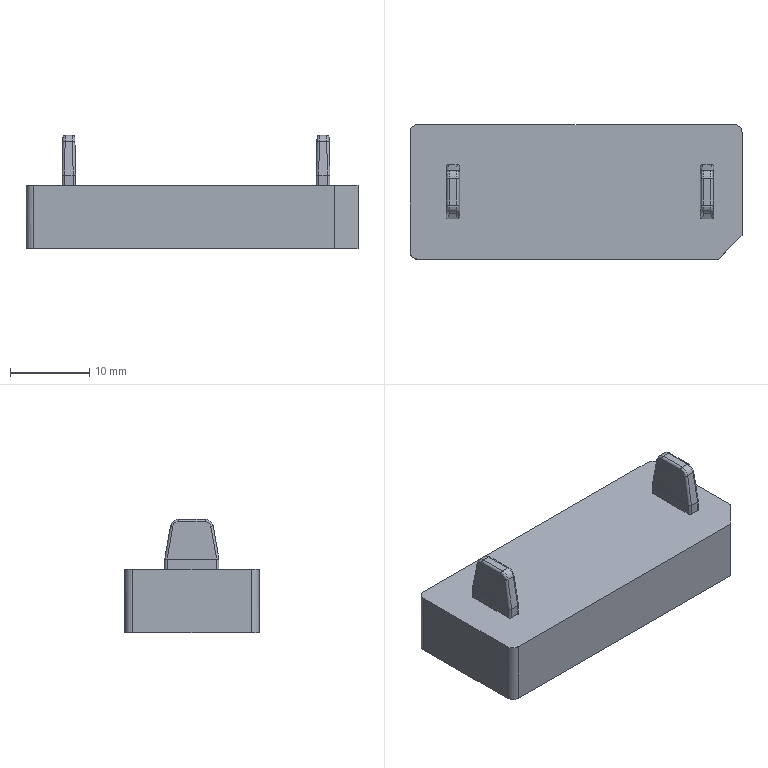CAM job | PowerMill | 3-axis milling, other | part box 42 x 17 x 14.346 mm
Tools:
number,name,type,diameter,tip_radius,length,cutting_length,overhang,flutes,holder,toolpaths_using
4,R1_2,ball_nosed,2.0,1.0,3.0,,2.0,1,D42L35,1
1,D10C_1_1,end_mill,10.0,0.0,60.0,,14.8,1,D42L35,6
3,D10_1_1,end_mill,10.0,0.0,60.0,,14.52,1,D42L35,6
4,R1_1_1,ball_nosed,2.0,1.0,3.0,,2.2,1,D42L35,1
5,B4R0.5_1_1,tip_radiused,4.0,0.5,30.0,,6.52,1,D42L35,1
13,Text_D4_1_1,taper_spherical,4.0,0.3,60.0,,6.6,1,D42L35,2
5,B4R0.5_2_1,tip_radiused,4.0,0.5,30.0,,6.4,1,D42L35,1
Operations:
program,toolpath,strategy,tool,tool_number,tool_diameter,tip_radius,flutes,spindle_rpm,feed_cut,surface_speed_m_min_computed,feed_per_tooth_computed,tolerance,thickness,stepover,stepdown,cut_length,cut_time_min,total_time_min,workplane
10-0804-1-F,精公开粗01-扫面平行-D10C,raster_area_clear,D10C_1_1,1,10.0,0.0,1.0,8000.0,10000.0,251.33,1.25,0.03,0.28,6.0,1.0,260.36,0.026,0.0323,
10-0804-1-F,精公开粗01-外形偏置-D10C,offset_area_clear,D10C_1_1,1,10.0,0.0,1.0,8000.0,10000.0,251.33,1.25,0.03,0.28,6.0,1.0,4731.472,0.473,0.5156,
10-0804-1-F,精公开粗01-基准台等高-D10C,constantz,D10C_1_1,1,10.0,0.0,1.0,8000.0,10000.0,251.33,1.25,0.03,0.07,5.0,0.4,3229.05,0.323,0.3318,
10-0804-1-F,精公基准台01-平坦面平行-D10,raster_area_clear,D10_1_1,3,10.0,0.0,1.0,8500.0,600.0,267.04,0.0706,0.005,0.38,5.0,1.0,63.666,0.106,0.1389,
10-0804-1-F,精公基准台01-基准面偏置-D10,offset_area_clear,D10_1_1,3,10.0,0.0,1.0,8500.0,600.0,267.04,0.0706,0.005,0.38,5.0,1.0,214.171,0.357,0.3951,
10-0804-1-F,精公基准台01-基准台侧光-D10,profile_area_clear,D10_1_1,3,10.0,0.0,1.0,8500.0,600.0,267.04,0.0706,0.005,0.0,0.08,1.0,293.234,0.489,0.5523,
10-0804-1-F,精公精光01-平行-R1,raster,R1_1_1,4,2.0,1.0,1.0,18000.0,2000.0,113.1,0.1111,0.005,-0.075,0.03,1.0,2199.166,1.1,1.119,
10-0804-1-F,精公精光02-等高-B4R0.5,constantz,B4R0.5_1_1,5,4.0,0.5,1.0,18000.0,2000.0,226.19,0.1111,0.005,-0.075,5.0,0.04,8408.765,4.204,4.217,
10-0804-1-F,精公刻字01-刻字-Text_D4,pattern,Text_D4_1_1,13,4.0,0.3,1.0,15000.0,1000.0,188.5,0.0667,0.005,0.0,5.0,1.0,59.894,0.06,0.0789,
10-0804-1-R,粗公开粗01-扫面平行-D10C,raster_area_clear,D10C_1_1,1,10.0,0.0,1.0,8000.0,10000.0,251.33,1.25,0.03,0.15,6.0,1.0,517.6,0.052,0.059,
10-0804-1-R,粗公开粗01-外形偏置-D10C,offset_area_clear,D10C_1_1,1,10.0,0.0,1.0,8000.0,10000.0,251.33,1.25,0.03,0.15,6.0,1.0,4688.354,0.469,0.5114,
10-0804-1-R,粗公开粗01-基准台等高-D10C,constantz,D10C_1_1,1,10.0,0.0,1.0,8000.0,10000.0,251.33,1.25,0.03,0.07,5.0,0.4,3229.05,0.323,0.3318,
10-0804-1-R,粗公基准台01-平坦面平行-D10,raster_area_clear,D10_1_1,3,10.0,0.0,1.0,8500.0,600.0,267.04,0.0706,0.01,0.25,5.0,1.0,62.783,0.105,0.1374,
10-0804-1-R,粗公基准台01-基准面偏置-D10,offset_area_clear,D10_1_1,3,10.0,0.0,1.0,8500.0,600.0,267.04,0.0706,0.01,0.25,5.0,1.0,212.11,0.353,0.3916,
10-0804-1-R,粗公基准台01-基准台侧光-D10,profile_area_clear,D10_1_1,3,10.0,0.0,1.0,8500.0,600.0,267.04,0.0706,0.01,0.0,0.08,1.0,293.217,0.489,0.5522,
10-0804-1-R,粗公精光01-平行-R1,raster,R1_2,4,2.0,1.0,1.0,18000.0,2000.0,113.1,0.1111,0.01,-0.205,0.036,1.0,1601.824,0.801,0.8202,
10-0804-1-R,粗公精光02-等高-B4R0.5,constantz,B4R0.5_2_1,5,4.0,0.5,1.0,18000.0,2000.0,226.19,0.1111,0.01,-0.205,5.0,0.048,6722.471,3.361,3.374,
10-0804-1-R,粗公刻字01-刻字-Text_D4,pattern,Text_D4_1_1,13,4.0,0.3,1.0,15000.0,1000.0,188.5,0.0667,0.01,0.0,5.0,1.0,56.507,0.057,0.0745,